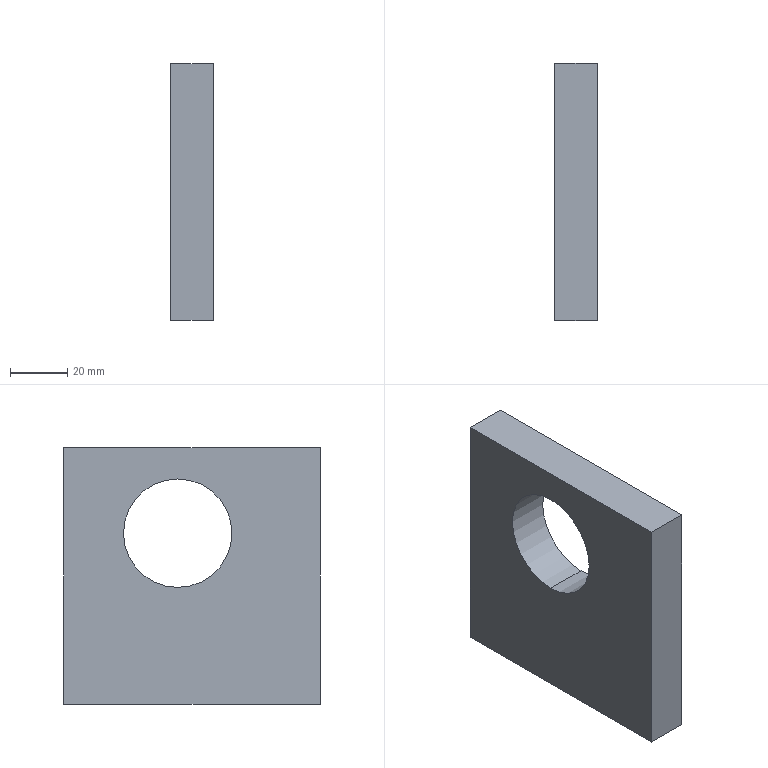Part | SolidWorks | features Extrusion 1, ICE 1 | 1 solid | 8 faces | box 15 x 90 x 90 mm | volume 104488 mm3 | plane 6 | cylinder 2 | commonest cylinder face diameters 38 x2
STEP:
#1=CARTESIAN_POINT('',(-7.5,5.,34.));
#2=VERTEX_POINT('',#1);
#3=CARTESIAN_POINT('',(-7.5,5.,-4.));
#4=VERTEX_POINT('',#3);
#5=CARTESIAN_POINT('',(-7.5,5.,15.));
#6=DIRECTION('',(1.,0.,0.));
#7=DIRECTION('',(0.,0.,-1.));
#8=AXIS2_PLACEMENT_3D('',#5,#6,#7);
#9=CIRCLE('',#8,19.);
#10=EDGE_CURVE('',#2,#4,#9,.T.);
#11=ORIENTED_EDGE('',*,*,#10,.F.);
#12=CARTESIAN_POINT('',(7.5,5.,34.));
#13=VERTEX_POINT('',#12);
#14=CARTESIAN_POINT('',(-7.5,5.,34.));
#15=DIRECTION('',(1.,0.,0.));
#16=VECTOR('',#15,1000.);
#17=LINE('',#14,#16);
#18=EDGE_CURVE('',#2,#13,#17,.T.);
#19=ORIENTED_EDGE('',*,*,#18,.T.);
#20=CARTESIAN_POINT('',(7.5,5.,-4.));
#21=VERTEX_POINT('',#20);
#22=CARTESIAN_POINT('',(7.5,5.,15.));
#23=DIRECTION('',(1.,0.,0.));
#24=DIRECTION('',(0.,0.,-1.));
#25=AXIS2_PLACEMENT_3D('',#22,#23,#24);
#26=CIRCLE('',#25,19.);
#27=EDGE_CURVE('',#13,#21,#26,.T.);
#28=ORIENTED_EDGE('',*,*,#27,.T.);
#29=CARTESIAN_POINT('',(-7.5,5.,-4.));
#30=DIRECTION('',(1.,0.,0.));
#31=VECTOR('',#30,1000.);
#32=LINE('',#29,#31);
#33=EDGE_CURVE('',#4,#21,#32,.T.);
#34=ORIENTED_EDGE('',*,*,#33,.F.);
#35=EDGE_LOOP('',(#11,#19,#28,#34));
#36=FACE_OUTER_BOUND('',#35,.T.);
#37=CARTESIAN_POINT('',(-7.5,5.,15.));
#38=DIRECTION('',(1.,0.,0.));
#39=DIRECTION('',(0.,0.,-1.));
#40=AXIS2_PLACEMENT_3D('',#37,#38,#39);
#41=CYLINDRICAL_SURFACE('',#40,19.);
#42=ADVANCED_FACE('',(#36),#41,.F.);
#43=CARTESIAN_POINT('',(-7.5,45.,45.));
#44=VERTEX_POINT('',#43);
#45=CARTESIAN_POINT('',(-7.5,-45.,45.));
#46=VERTEX_POINT('',#45);
#47=CARTESIAN_POINT('',(-7.5,-45.,45.));
#48=DIRECTION('',(0.,-1.,0.));
#49=VECTOR('',#48,1000.);
#50=LINE('',#47,#49);
#51=EDGE_CURVE('',#44,#46,#50,.T.);
#52=ORIENTED_EDGE('',*,*,#51,.T.);
#53=CARTESIAN_POINT('',(7.5,-45.,45.));
#54=VERTEX_POINT('',#53);
#55=CARTESIAN_POINT('',(7.5,-45.,45.));
#56=DIRECTION('',(-1.,0.,0.));
#57=VECTOR('',#56,1000.);
#58=LINE('',#55,#57);
#59=EDGE_CURVE('',#54,#46,#58,.T.);
#60=ORIENTED_EDGE('',*,*,#59,.F.);
#61=CARTESIAN_POINT('',(7.5,45.,45.));
#62=VERTEX_POINT('',#61);
#63=CARTESIAN_POINT('',(7.5,-45.,45.));
#64=DIRECTION('',(0.,-1.,0.));
#65=VECTOR('',#64,1000.);
#66=LINE('',#63,#65);
#67=EDGE_CURVE('',#62,#54,#66,.T.);
#68=ORIENTED_EDGE('',*,*,#67,.F.);
#69=CARTESIAN_POINT('',(7.5,45.,45.));
#70=DIRECTION('',(-1.,0.,0.));
#71=VECTOR('',#70,1000.);
#72=LINE('',#69,#71);
#73=EDGE_CURVE('',#62,#44,#72,.T.);
#74=ORIENTED_EDGE('',*,*,#73,.T.);
#75=EDGE_LOOP('',(#52,#60,#68,#74));
#76=FACE_OUTER_BOUND('',#75,.T.);
#77=CARTESIAN_POINT('',(7.5,-45.,45.));
#78=DIRECTION('',(0.,0.,-1.));
#79=DIRECTION('',(-1.,0.,0.));
#80=AXIS2_PLACEMENT_3D('',#77,#78,#79);
#81=PLANE('',#80);
#82=ADVANCED_FACE('',(#76),#81,.F.);
#83=CARTESIAN_POINT('',(-7.5,-45.,-45.));
#84=VERTEX_POINT('',#83);
#85=CARTESIAN_POINT('',(-7.5,-45.,-45.));
#86=DIRECTION('',(0.,0.,-1.));
#87=VECTOR('',#86,1000.);
#88=LINE('',#85,#87);
#89=EDGE_CURVE('',#46,#84,#88,.T.);
#90=ORIENTED_EDGE('',*,*,#89,.T.);
#91=CARTESIAN_POINT('',(7.5,-45.,-45.));
#92=VERTEX_POINT('',#91);
#93=CARTESIAN_POINT('',(7.5,-45.,-45.));
#94=DIRECTION('',(-1.,0.,0.));
#95=VECTOR('',#94,1000.);
#96=LINE('',#93,#95);
#97=EDGE_CURVE('',#92,#84,#96,.T.);
#98=ORIENTED_EDGE('',*,*,#97,.F.);
#99=CARTESIAN_POINT('',(7.5,-45.,-45.));
#100=DIRECTION('',(0.,0.,-1.));
#101=VECTOR('',#100,1000.);
#102=LINE('',#99,#101);
#103=EDGE_CURVE('',#54,#92,#102,.T.);
#104=ORIENTED_EDGE('',*,*,#103,.F.);
#105=ORIENTED_EDGE('',*,*,#59,.T.);
#106=EDGE_LOOP('',(#90,#98,#104,#105));
#107=FACE_OUTER_BOUND('',#106,.T.);
#108=CARTESIAN_POINT('',(7.5,-45.,-45.));
#109=DIRECTION('',(0.,1.,0.));
#110=DIRECTION('',(0.,0.,1.));
#111=AXIS2_PLACEMENT_3D('',#108,#109,#110);
#112=PLANE('',#111);
#113=ADVANCED_FACE('',(#107),#112,.F.);
#114=CARTESIAN_POINT('',(-7.5,45.,-45.));
#115=VERTEX_POINT('',#114);
#116=CARTESIAN_POINT('',(-7.5,-45.,-45.));
#117=DIRECTION('',(0.,1.,0.));
#118=VECTOR('',#117,1000.);
#119=LINE('',#116,#118);
#120=EDGE_CURVE('',#84,#115,#119,.T.);
#121=ORIENTED_EDGE('',*,*,#120,.T.);
#122=CARTESIAN_POINT('',(7.5,45.,-45.));
#123=VERTEX_POINT('',#122);
#124=CARTESIAN_POINT('',(7.5,45.,-45.));
#125=DIRECTION('',(-1.,0.,0.));
#126=VECTOR('',#125,1000.);
#127=LINE('',#124,#126);
#128=EDGE_CURVE('',#123,#115,#127,.T.);
#129=ORIENTED_EDGE('',*,*,#128,.F.);
#130=CARTESIAN_POINT('',(7.5,-45.,-45.));
#131=DIRECTION('',(0.,1.,0.));
#132=VECTOR('',#131,1000.);
#133=LINE('',#130,#132);
#134=EDGE_CURVE('',#92,#123,#133,.T.);
#135=ORIENTED_EDGE('',*,*,#134,.F.);
#136=ORIENTED_EDGE('',*,*,#97,.T.);
#137=EDGE_LOOP('',(#121,#129,#135,#136));
#138=FACE_OUTER_BOUND('',#137,.T.);
#139=CARTESIAN_POINT('',(7.5,-45.,-45.));
#140=DIRECTION('',(0.,0.,1.));
#141=DIRECTION('',(1.,0.,0.));
#142=AXIS2_PLACEMENT_3D('',#139,#140,#141);
#143=PLANE('',#142);
#144=ADVANCED_FACE('',(#138),#143,.F.);
#145=CARTESIAN_POINT('',(-7.5,45.,-45.));
#146=DIRECTION('',(0.,0.,1.));
#147=VECTOR('',#146,1000.);
#148=LINE('',#145,#147);
#149=EDGE_CURVE('',#115,#44,#148,.T.);
#150=ORIENTED_EDGE('',*,*,#149,.T.);
#151=ORIENTED_EDGE('',*,*,#73,.F.);
#152=CARTESIAN_POINT('',(7.5,45.,-45.));
#153=DIRECTION('',(0.,0.,1.));
#154=VECTOR('',#153,1000.);
#155=LINE('',#152,#154);
#156=EDGE_CURVE('',#123,#62,#155,.T.);
#157=ORIENTED_EDGE('',*,*,#156,.F.);
#158=ORIENTED_EDGE('',*,*,#128,.T.);
#159=EDGE_LOOP('',(#150,#151,#157,#158));
#160=FACE_OUTER_BOUND('',#159,.T.);
#161=CARTESIAN_POINT('',(7.5,45.,-45.));
#162=DIRECTION('',(0.,-1.,0.));
#163=DIRECTION('',(0.,0.,-1.));
#164=AXIS2_PLACEMENT_3D('',#161,#162,#163);
#165=PLANE('',#164);
#166=ADVANCED_FACE('',(#160),#165,.F.);
#167=CARTESIAN_POINT('',(7.5,5.,15.));
#168=DIRECTION('',(1.,0.,0.));
#169=DIRECTION('',(0.,0.,-1.));
#170=AXIS2_PLACEMENT_3D('',#167,#168,#169);
#171=CIRCLE('',#170,19.);
#172=EDGE_CURVE('',#21,#13,#171,.T.);
#173=ORIENTED_EDGE('',*,*,#172,.F.);
#174=ORIENTED_EDGE('',*,*,#27,.F.);
#175=EDGE_LOOP('',(#173,#174));
#176=FACE_BOUND('',#175,.T.);
#177=ORIENTED_EDGE('',*,*,#67,.T.);
#178=ORIENTED_EDGE('',*,*,#103,.T.);
#179=ORIENTED_EDGE('',*,*,#134,.T.);
#180=ORIENTED_EDGE('',*,*,#156,.T.);
#181=EDGE_LOOP('',(#177,#178,#179,#180));
#182=FACE_OUTER_BOUND('',#181,.T.);
#183=CARTESIAN_POINT('',(7.5,0.,0.));
#184=DIRECTION('',(1.,0.,0.));
#185=DIRECTION('',(0.,0.,-1.));
#186=AXIS2_PLACEMENT_3D('',#183,#184,#185);
#187=PLANE('',#186);
#188=ADVANCED_FACE('',(#176,#182),#187,.T.);
#189=CARTESIAN_POINT('',(-7.5,5.,15.));
#190=DIRECTION('',(1.,0.,0.));
#191=DIRECTION('',(0.,0.,-1.));
#192=AXIS2_PLACEMENT_3D('',#189,#190,#191);
#193=CIRCLE('',#192,19.);
#194=EDGE_CURVE('',#4,#2,#193,.T.);
#195=ORIENTED_EDGE('',*,*,#194,.T.);
#196=ORIENTED_EDGE('',*,*,#10,.T.);
#197=EDGE_LOOP('',(#195,#196));
#198=FACE_BOUND('',#197,.T.);
#199=ORIENTED_EDGE('',*,*,#51,.F.);
#200=ORIENTED_EDGE('',*,*,#149,.F.);
#201=ORIENTED_EDGE('',*,*,#120,.F.);
#202=ORIENTED_EDGE('',*,*,#89,.F.);
#203=EDGE_LOOP('',(#199,#200,#201,#202));
#204=FACE_OUTER_BOUND('',#203,.T.);
#205=CARTESIAN_POINT('',(-7.5,0.,0.));
#206=DIRECTION('',(1.,0.,0.));
#207=DIRECTION('',(0.,0.,-1.));
#208=AXIS2_PLACEMENT_3D('',#205,#206,#207);
#209=PLANE('',#208);
#210=ADVANCED_FACE('',(#198,#204),#209,.F.);
#211=ORIENTED_EDGE('',*,*,#18,.F.);
#212=ORIENTED_EDGE('',*,*,#194,.F.);
#213=ORIENTED_EDGE('',*,*,#33,.T.);
#214=ORIENTED_EDGE('',*,*,#172,.T.);
#215=EDGE_LOOP('',(#211,#212,#213,#214));
#216=FACE_OUTER_BOUND('',#215,.T.);
#217=CARTESIAN_POINT('',(-7.5,5.,15.));
#218=DIRECTION('',(1.,0.,0.));
#219=DIRECTION('',(0.,0.,-1.));
#220=AXIS2_PLACEMENT_3D('',#217,#218,#219);
#221=CYLINDRICAL_SURFACE('',#220,19.);
#222=ADVANCED_FACE('',(#216),#221,.F.);
#223=CLOSED_SHELL('',(#42,#82,#113,#144,#166,#188,#210,#222));
#224=MANIFOLD_SOLID_BREP('',#223);
#225=CARTESIAN_POINT('',(0.,0.,0.));
#226=DIRECTION('',(0.,0.,1.));
#227=DIRECTION('',(1.,0.,0.));
#228=AXIS2_PLACEMENT_3D('',#225,#226,#227);
#229=(LENGTH_UNIT()NAMED_UNIT(*)SI_UNIT(.MILLI.,.METRE.));
#230=UNCERTAINTY_MEASURE_WITH_UNIT(LENGTH_MEASURE(0.00001),#229,'','');
#231=(NAMED_UNIT(*)PLANE_ANGLE_UNIT()SI_UNIT($,.RADIAN.));
#232=(NAMED_UNIT(*)SI_UNIT($,.STERADIAN.)SOLID_ANGLE_UNIT());
#233=(GEOMETRIC_REPRESENTATION_CONTEXT(3)GLOBAL_UNCERTAINTY_ASSIGNED_CONTEXT((#230))GLOBAL_UNIT_ASSIGNED_CONTEXT((#229,#231,#232))REPRESENTATION_CONTEXT('',''));
#234=ADVANCED_BREP_SHAPE_REPRESENTATION('',(#224,#228),#233);